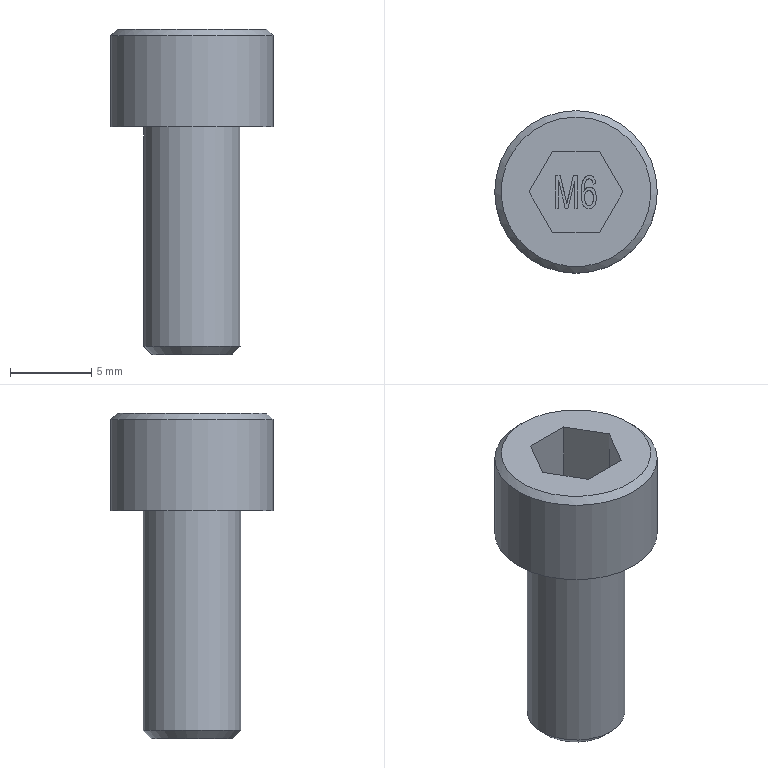Part | STEP file | EM10601400 | 1 solid | 38 faces | box 10 x 10 x 20 mm | volume 775.654 mm3 | plane 25 | other 9 | cylinder 2 | cone 2 | commonest cylinder face diameters 6 x1 10 x1